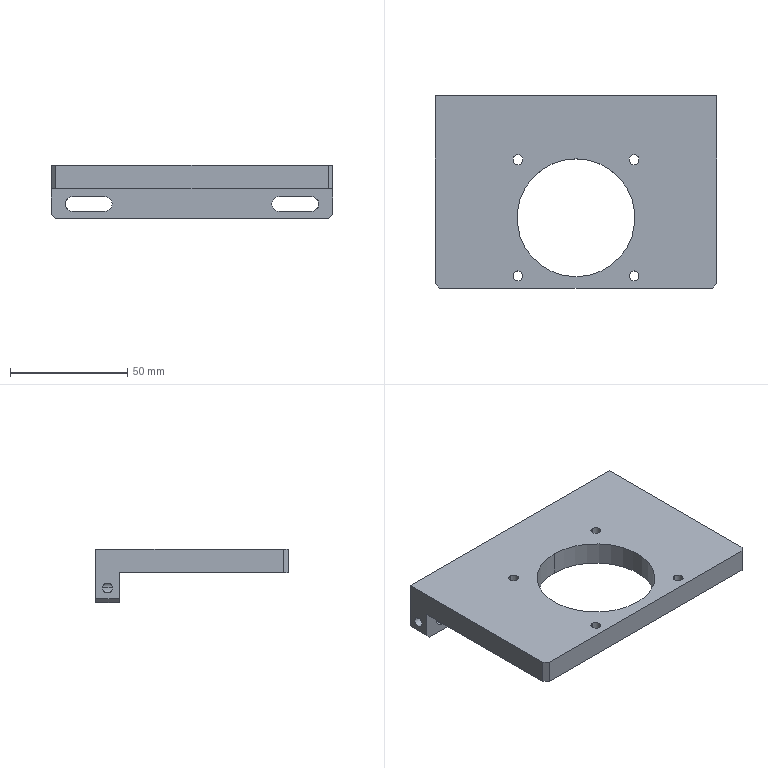NC program | NX | posted with a generic post | part box 120 x 82 x 22.8 mm
Lines 3184 to 3479 of 3479:
(ZLEVEL_PROFILE_1 , TOOL : D10JING)
N6354 T14 M6
N6356 G54
N6358 G17 G0 G90 X-61.622 Y47.809 B0. C0. S9500 M3
N6360 G43 Z30. H14
N6362 Z-9.9
N6364 G94 G1 Z-11.4 F1000.
N6366 X-60.866 Y46.5
N6368 G3 X-60. Y46. R1.
N6370 G1 X60. F1500.
N6372 G2 X65. Y41. R5.
N6374 G1 Y-39.
N6376 G2 X63.536 Y-42.536 R5.
N6378 G1 X61.536 Y-44.536
N6380 G2 X58. Y-46. R5.
N6382 G1 X-58.
N6384 G2 X-61.536 Y-44.536 R5.
N6386 G1 X-63.536 Y-42.536
N6388 G2 X-65. Y-39. R5.
N6390 G1 Y41.
N6392 G2 X-60. Y46. R5.
N6394 G1 X60. Z-14.559
N6396 X60.49 Y45.976 Z-14.572
N6398 X60.975 Y45.904 Z-14.585
N6400 X61.451 Y45.785 Z-14.598
N6402 X61.913 Y45.619 Z-14.611
N6404 X62.357 Y45.41 Z-14.624
N6406 X62.778 Y45.157 Z-14.637
N6408 X63.172 Y44.865 Z-14.65
N6410 X63.536 Y44.536 Z-14.662
N6412 X63.865 Y44.172 Z-14.675
N6414 X64.157 Y43.778 Z-14.688
N6416 X64.41 Y43.357 Z-14.701
N6418 X64.619 Y42.913 Z-14.714
N6420 X64.785 Y42.451 Z-14.727
N6422 X64.904 Y41.975 Z-14.74
N6424 X64.976 Y41.49 Z-14.753
N6426 X65. Y41. Z-14.766
N6428 Y-39. Z-16.872
N6430 X64.976 Y-39.49 Z-16.885
N6432 X64.904 Y-39.975 Z-16.898
N6434 X64.785 Y-40.451 Z-16.91
N6436 X64.619 Y-40.913 Z-16.923
N6438 X64.41 Y-41.357 Z-16.936
N6440 X64.157 Y-41.778 Z-16.949
N6442 X63.865 Y-42.172 Z-16.962
N6444 X63.536 Y-42.536 Z-16.975
N6446 X61.536 Y-44.536 Z-17.049
N6448 X61.172 Y-44.865 Z-17.062
N6450 X60.778 Y-45.157 Z-17.075
N6452 X60.357 Y-45.41 Z-17.088
N6454 X59.913 Y-45.619 Z-17.101
N6456 X59.451 Y-45.785 Z-17.114
N6458 X58.975 Y-45.904 Z-17.127
N6460 X58.49 Y-45.976 Z-17.14
N6462 X58. Y-46. Z-17.153
N6464 X-58. Z-20.207
N6466 X-58.49 Y-45.976 Z-20.219
N6468 X-58.975 Y-45.904 Z-20.232
N6470 X-59.451 Y-45.785 Z-20.245
N6472 X-59.913 Y-45.619 Z-20.258
N6474 X-60.357 Y-45.41 Z-20.271
N6476 X-60.778 Y-45.157 Z-20.284
N6478 X-61.172 Y-44.865 Z-20.297
N6480 X-61.536 Y-44.536 Z-20.31
N6482 X-63.536 Y-42.536 Z-20.384
N6484 X-63.865 Y-42.172 Z-20.397
N6486 X-64.157 Y-41.778 Z-20.41
N6488 X-64.41 Y-41.357 Z-20.423
N6490 X-64.619 Y-40.913 Z-20.436
N6492 X-64.785 Y-40.451 Z-20.449
N6494 X-64.904 Y-39.975 Z-20.462
N6496 X-64.976 Y-39.49 Z-20.475
N6498 X-65. Y-39. Z-20.487
N6500 Y41. Z-22.594
N6502 X-64.976 Y41.49 Z-22.606
N6504 X-64.904 Y41.975 Z-22.619
N6506 X-64.785 Y42.451 Z-22.632
N6508 X-64.619 Y42.913 Z-22.645
N6510 X-64.41 Y43.357 Z-22.658
N6512 X-64.157 Y43.778 Z-22.671
N6514 X-63.865 Y44.172 Z-22.684
N6516 X-63.536 Y44.536 Z-22.697
N6518 X-63.172 Y44.865 Z-22.71
N6520 X-62.778 Y45.157 Z-22.723
N6522 X-62.357 Y45.41 Z-22.735
N6524 X-61.913 Y45.619 Z-22.748
N6526 X-61.451 Y45.785 Z-22.761
N6528 X-60.975 Y45.904 Z-22.774
N6530 X-60.49 Y45.976 Z-22.787
N6532 X-60. Y46. Z-22.8
N6534 X60.
N6536 G2 X65. Y41. R5.
N6538 G1 Y-39.
N6540 G2 X63.536 Y-42.536 R5.
N6542 G1 X61.536 Y-44.536
N6544 G2 X58. Y-46. R5.
N6546 G1 X-58.
N6548 G2 X-61.536 Y-44.536 R5.
N6550 G1 X-63.536 Y-42.536
N6552 G2 X-65. Y-39. R5.
N6554 G1 Y41.
N6556 G2 X-60. Y46. R5.
N6558 G3 X-59.134 Y46.5 R1.
N6560 G1 X-58.268 Y48.
N6562 Z-21.3
N6564 G0 Z30.
(ZLEVEL_PROFILE_1_COPY , TOOL : D10JING)
N6566 X20.002 Y-9.308
N6568 Z1.5
N6570 G1 X19.804 Y-7.391 Z1.399 F1000.
N6572 X19.015 Y-4.393 Z1.237
N6574 X18.182 Y-2.36 Z1.121
N6576 X16.652 Y0.311 Z0.96
N6578 X14.733 Y2.717 Z0.799
N6580 X12.469 Y4.803 Z0.637
N6582 X9.914 Y6.519 Z0.476
N6584 X7.127 Y7.826 Z0.315
N6586 X4.174 Y8.693 Z0.154
N6588 X1.123 Y9.099 Z-0.008
N6590 X-1.074 Y9.101 Z-0.123
N6592 X-4.151 Y8.697 Z-0.286
N6594 X-7.13 Y7.825 Z-0.448
N6596 X-9.938 Y6.506 Z-0.611
N6598 X-12.511 Y4.77 Z-0.773
N6600 X-14.786 Y2.66 Z-0.936
N6602 X-16.71 Y0.225 Z-1.099
N6604 X-18.237 Y-2.477 Z-1.261
N6606 X-19.33 Y-5.381 Z-1.424
N6608 X-19.964 Y-8.419 Z-1.587
N6610 X-20.123 Y-11.518 Z-1.749
N6612 X-19.805 Y-14.605 Z-1.912
N6614 X-19.015 Y-17.607 Z-2.075
N6616 X-18.182 Y-19.64 Z-2.19
N6618 X-16.65 Y-22.313 Z-2.351
N6620 X-14.728 Y-24.722 Z-2.513
N6622 X-12.461 Y-26.809 Z-2.674
N6624 X-9.902 Y-28.526 Z-2.836
N6626 X-7.111 Y-29.832 Z-2.997
N6628 X-4.154 Y-30.697 Z-3.159
N6630 X-1.099 Y-31.1 Z-3.32
N6632 X0.024 Z-3.379
N6634 X1.123 Y-31.099 Z-3.437
N6636 X4.195 Y-30.688 Z-3.599
N6638 X7.167 Y-29.811 Z-3.761
N6640 X9.97 Y-28.488 Z-3.924
N6642 X12.536 Y-26.75 Z-4.086
N6644 X14.805 Y-24.639 Z-4.249
N6646 X16.723 Y-22.205 Z-4.411
N6648 X18.245 Y-19.505 Z-4.574
N6650 X19.334 Y-16.603 Z-4.736
N6652 X19.965 Y-13.569 Z-4.898
N6654 X20.123 Y-10.473 Z-5.061
N6656 X19.804 Y-7.391 Z-5.223
N6658 X19.015 Y-4.393 Z-5.386
N6660 X18.182 Y-2.36 Z-5.501
N6662 X16.652 Y0.311 Z-5.662
N6664 X14.733 Y2.717 Z-5.823
N6666 X12.469 Y4.803 Z-5.985
N6668 X9.914 Y6.519 Z-6.146
N6670 X7.127 Y7.826 Z-6.307
N6672 X4.174 Y8.693 Z-6.469
N6674 X1.123 Y9.099 Z-6.63
N6676 X-1.074 Y9.101 Z-6.745
N6678 X-4.151 Y8.697 Z-6.908
N6680 X-7.13 Y7.825 Z-7.07
N6682 X-9.938 Y6.506 Z-7.233
N6684 X-12.511 Y4.77 Z-7.396
N6686 X-14.786 Y2.66 Z-7.558
N6688 X-16.71 Y0.225 Z-7.721
N6690 X-18.237 Y-2.477 Z-7.884
N6692 X-19.33 Y-5.381 Z-8.046
N6694 X-19.964 Y-8.419 Z-8.209
N6696 X-20.123 Y-11.518 Z-8.372
N6698 X-19.805 Y-14.605 Z-8.534
N6700 X-19.015 Y-17.607 Z-8.697
N6702 X-18.182 Y-19.64 Z-8.812
N6704 X-16.65 Y-22.313 Z-8.973
N6706 X-14.728 Y-24.722 Z-9.135
N6708 X-12.461 Y-26.809 Z-9.296
N6710 X-9.902 Y-28.526 Z-9.458
N6712 X-7.111 Y-29.832 Z-9.619
N6714 X-4.154 Y-30.697 Z-9.781
N6716 X-1.099 Y-31.1 Z-9.942
N6718 X0. Z-10.
N6720 X0.024 F1500.
N6722 G3 X20.1 Y-10.976 R20.1
N6724 X0. Y-31.1 R-20.1
N6726 G1 Z-8.5
N6728 G0 Z30.
N6730 M5
(DRILLING , TOOL : D6A45)
N6732 T01 M6
N6734 G54
N6736 G17 G0 G90 X-24.749 Y-35.749 B0. C0. S9500 M3
N6738 G43 Z30. H1
N6740 G94 G81 G98 Z-1. F250. R3.
N6742 X24.749
N6744 X-24.749 Y13.749
N6746 X24.749
N6748 G80
N6750 G0 X24.749 Y13.749 Z30.
N6752 M5
(DRILLING_COPY_COPY , TOOL : 4.2ZT)
N6754 T04 M6
N6756 G54
N6758 G17 G0 G90 X-24.749 Y-35.749 B0. C0. S2000 M3
N6760 G43 Z30. H4
N6762 G94 G83 G98 Z-12.762 F150. Q2. R3.
N6764 Y13.749
N6766 X24.749
N6768 Y-35.749
N6770 G80
N6772 G0 X24.749 Y-35.749 Z30.
N6774 M5
(PLANAR_MILL , TOOL : D6A45)
N6776 T01 M6
N6778 G54
N6780 G17 G0 G90 X23.883 Y-36.449 B0. C0. S9500 M3
N6782 G43 Z30. H1
N6784 Z0.5
N6786 G94 G1 Z-1. F1250.
N6788 G3 X24.749 Y-36.949 R1.
N6790 X25.949 Y-35.749 R1.2
N6792 X24.749 Y-36.949 R-1.2
N6794 X25.615 Y-36.449 R1.
N6796 G1 Z0.5
N6798 G0 Z30.
N6800 X-0.866 Y-34.7
N6802 Z0.5
N6804 G1 Z-1.
N6806 G3 X0. Y-35.2 R1.
N6808 X24.2 Y-11. R24.2
N6810 X0. Y-35.2 R-24.2
N6812 X0.866 Y-34.7 R1.
N6814 G1 Z0.5
N6816 G0 Z30.
N6818 X25.615 Y14.449
N6820 Z0.5
N6822 G1 Z-1.
N6824 G3 X24.749 Y14.949 R1.
N6826 X23.549 Y13.749 R1.2
N6828 X24.749 Y14.949 R-1.2
N6830 X23.883 Y14.449 R1.
N6832 G1 Z0.5
N6834 G0 Z30.
N6836 X-0.866 Y42.4
N6838 Z0.5
N6840 G1 Z-1.
N6842 G3 X0. Y41.9 R1.
N6844 G1 X60.
N6846 G2 X60.9 Y41. R0.9
N6848 G1 Y-39.
N6850 G2 X60.636 Y-39.636 R0.9
N6852 G1 X58.636 Y-41.636
N6854 G2 X58. Y-41.9 R0.9
N6856 G1 X-58.
N6858 G2 X-58.636 Y-41.636 R0.9
N6860 G1 X-60.636 Y-39.636
N6862 G2 X-60.9 Y-39. R0.9
N6864 G1 Y41.
N6866 G2 X-60. Y41.9 R0.9
N6868 G1 X0.
N6870 G3 X0.866 Y42.4 R1.
N6872 G1 Z0.5
N6874 G0 Z30.
N6876 X-23.883 Y14.449
N6878 Z0.5
N6880 G1 Z-1.
N6882 G3 X-24.749 Y14.949 R1.
N6884 X-25.949 Y13.749 R1.2
N6886 X-24.749 Y14.949 R-1.2
N6888 X-25.615 Y14.449 R1.
N6890 G1 Z0.5
N6892 G0 Z30.
N6894 Y-36.449
N6896 Z0.5
N6898 G1 Z-1.
N6900 G3 X-24.749 Y-36.949 R1.
N6902 X-23.549 Y-35.749 R1.2
N6904 X-24.749 Y-36.949 R-1.2
N6906 X-23.883 Y-36.449 R1.
N6908 G1 Z0.5
N6910 G0 Z30.
N6912 M5
N6914 M2